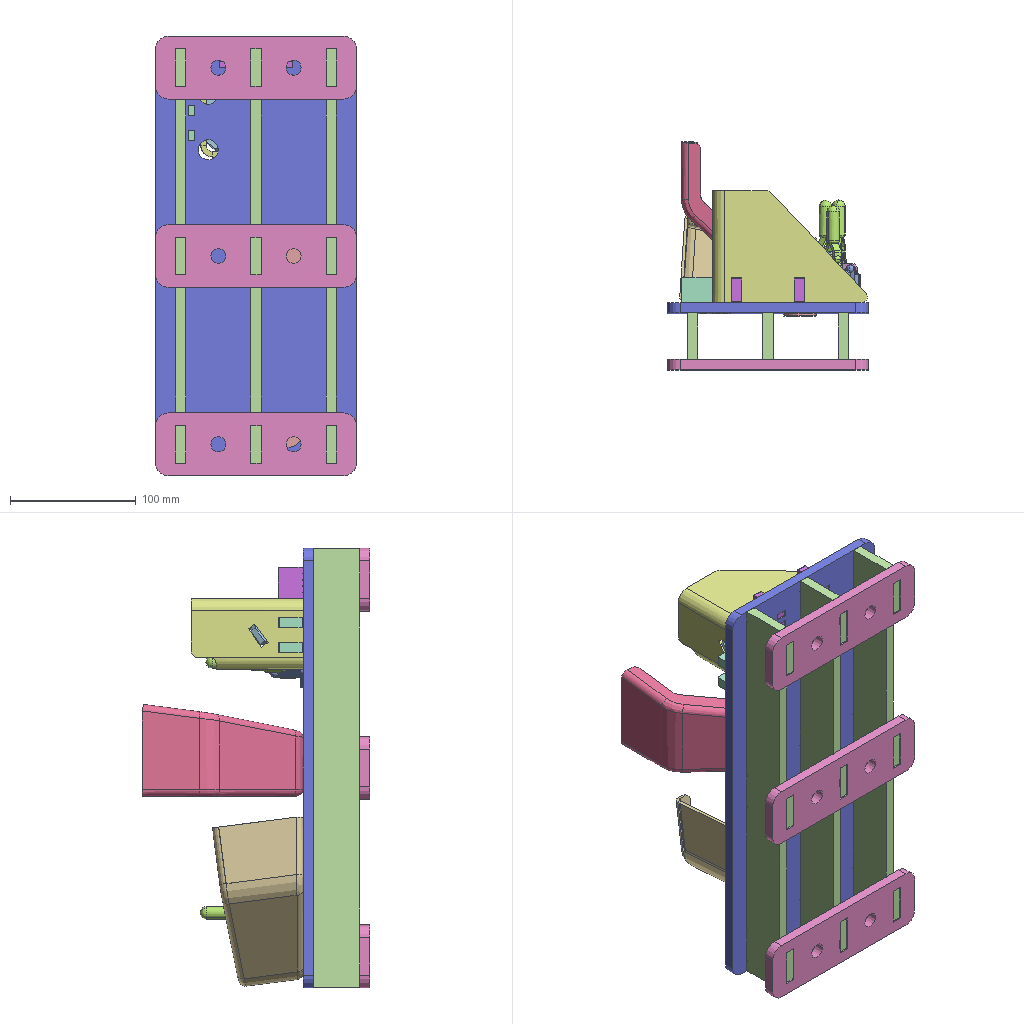Assembly | SolidWorks | 16 different items | 26 placed | box 160 x 181 x 350 mm
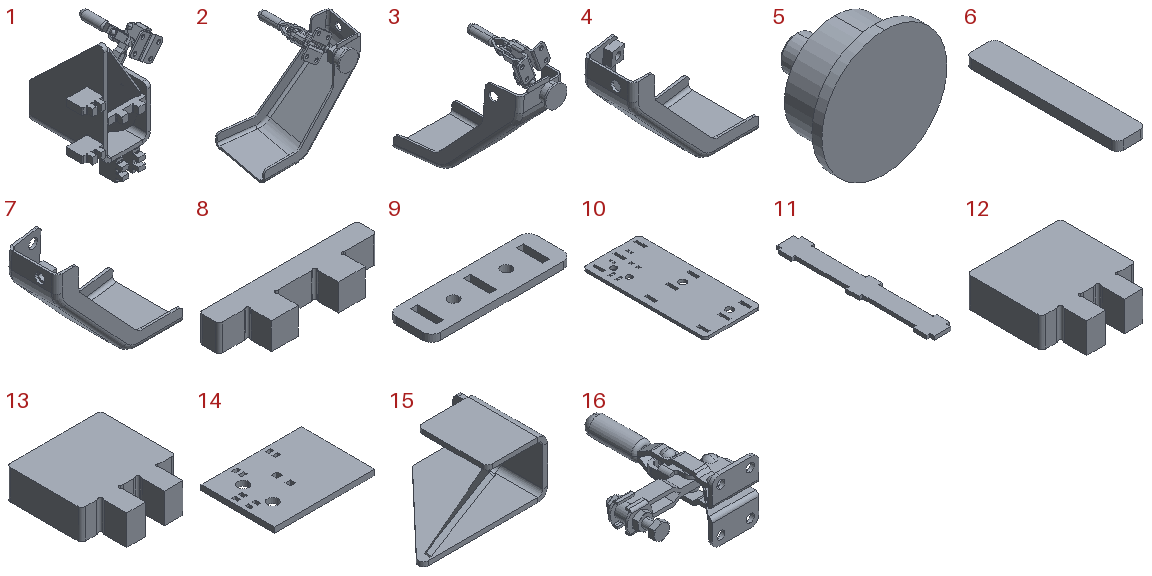Parts list (item | name | quantity | parent item | size | volume | features):
1 | (subassembly) | x1 | - | 95.955 x 96.4 x 148.047 mm | 120880 mm3 | features LocalLPattern 2, ReferencePattern 2
2 | (subassembly) | x1 | - | 134.657 x 92.265 x 136.571 mm | 37009 mm3 | -
3 | (subassembly) | x1 | - | 72.927 x 138.4 x 143.686 mm | 52890 mm3 | -
4 | - | x1 | in 2 | - | - | features MBimport 1
5 | - | x2 | in 2, 3 | 25 x 17.8 x 25 mm | 3845 mm3 | features Chamfer 1, Revolution 1
6 | - | x2 | in 2, 3 | 5 x 26 x 1.6 mm | 206.627 mm3 | features Fillet 1, FlatPattern 1, SMBaseFlange 1, SheetMetal 1
7 | - | x1 | in 3 | 128.4 x 72.927 x 105.583 mm | 38422 mm3 | features MBimport 1
8 | - | x1 | in 1 | 47.1 x 13 x 8 mm | 3140 mm3 | features Fillet 1, FlatPattern 1, ICE 1, SMBaseFlange 1, SheetMetal 1
9 | - | x3 | - | 160 x 50 x 8 mm | 55744 mm3 | features Fillet 1, FlatPattern 1, SMBaseFlange 1, SheetMetal 1
10 | - | x1 | - | 160 x 350 x 8 mm | 418206 mm3 | features Fillet 1, FlatPattern 1, SMBaseFlange 1, SheetMetal 1
11 | - | x3 | - | 51.5 x 350 x 8 mm | 114010 mm3 | features Fillet 1, FlatPattern 1, ICE 1, SMBaseFlange 1, SheetMetal 1
12 | - | x2 | in 1 | 25 x 27 x 8 mm | 4541 mm3 | features Fillet 1, FlatPattern 1, ICE 1, SMBaseFlange 1, SheetMetal 1
13 | - | x2 | in 1 | 25 x 27 x 8 mm | 4541 mm3 | features Fillet 1, FlatPattern 1, ICE 1, SMBaseFlange 1, SheetMetal 1
14 | - | x1 | in 1 | 150 x 110 x 8 mm | 125199 mm3 | features FlatPattern 1, SMBaseFlange 1, SheetMetal 1
15 | - | x1 | in 1 | 123.265 x 89.4 x 56.1 mm | 89195 mm3 | features MBimport 1
16 | - | x3 | in 1, 2, 3 | 56.45 x 77.62 x 33.3 mm | 10418 mm3 | features BaseBody 5
Mates (type | each side: item.copy, entity, surface, feature):
In the top assembly
Coincident | 5.1 face plane Revolve8 | 5.2 face plane Revolve8
Coincident | 6.1 face plane Base-Flange1 | 6.2 face plane Base-Flange1
DistanceDim | 5.1 face cylinder Revolve8 | 5.2 face cylinder Revolve8
InPlace | 3.1 face plane 2a5-53-11k61-SUB4.STEP | 10.1 plane
Coincident | 7.1 face plane 2a5-53-11k61-SUB4.STEP | 15.1 face plane 2a5-53-11k61-SUB1.STEP
DistanceDim | 6.2 face plane Base-Flange1 | 15.1 face plane 2a5-53-11k61-SUB1.STEP
DistanceDim | 6.2 face plane Base-Flange1 | 12.1 face plane Base-Flange1
InPlace | 10.1 face plane Base-Flange1 | 11.1 plane
InPlace | 11.2 face plane Base-Flange1 | 9.1 plane
In subassembly 2
Coincident | 5.3 face plane Revolve8 | 4.1 face plane 2a5-53-11k61-SUB3.STEP
Concentric | 5.3 face cylinder Revolve8 | 4.1 face cylinder 2a5-53-11k61-SUB3.STEP
Coincident | 4.1 face plane 2a5-53-11k61-SUB3.STEP | 16.1 face plane PN_0001 vertical flange-seat quick clamp [PN_0002].step-1/_PN_0001(bolt).step-1-solid1
Concentric | 4.1 face cylinder 2a5-53-11k61-SUB3.STEP | 16.1 face cylinder PN_0001 vertical flange-seat quick clamp [PN_0002].step-1/_PN_0001(bolt).step-1-solid1
PlanarAngleDim | 4.1 face plane 2a5-53-11k61-SUB3.STEP | 16.1 face plane PN_0001 vertical flange-seat quick clamp [PN_0002].step-1/_PN_0001(seat).step-1-solid1
Coincident | 4.1 face plane 2a5-53-11k61-SUB3.STEP | 6.3 face plane Base-Flange1 | 2 times
Parallel | 5.3 plane | 4.1 face plane 2a5-53-11k61-SUB3.STEP
Coincident | 4.1 vertex | 6.3 vertex
In subassembly 3
InPlace | 5.3 plane | 3.2 plane
Concentric | 7.2 face cylinder 2a5-53-11k61-SUB4.STEP | 16.1 face cylinder PN_0001 vertical flange-seat quick clamp [PN_0002].step-1/_PN_0001(bolt).step-1-solid1
Coincident | 7.2 face plane 2a5-53-11k61-SUB4.STEP | 16.1 face plane PN_0001 vertical flange-seat quick clamp [PN_0002].step-1/_PN_0001(bolt).step-1-solid1
PlanarAngleDim | 16.1 face plane PN_0001 vertical flange-seat quick clamp [PN_0002].step-1/_PN_0001(seat).step-1-solid1 | 7.2 face plane 2a5-53-11k61-SUB4.STEP
InPlace | 7.2 face plane 2a5-53-11k61-SUB4.STEP | 6.3 plane
In subassembly 1
InPlace | 12.2 plane | 1.1 plane
InPlace | 13.1 plane | 1.1 plane
Coincident | 15.2 face plane 2a5-53-11k61-SUB1.STEP | 16.1 face plane PN_0001 vertical flange-seat quick clamp [PN_0002].step-1/_PN_0001(seat).step-1-solid1
InPlace | 8.1 plane | 1.1 plane
Coincident | 15.2 face plane 2a5-53-11k61-SUB1.STEP | 14.1 face plane Base-Flange1
Coincident | 12.3 face plane Base-Flange1 | 14.1 face plane Base-Flange1 | 2 times